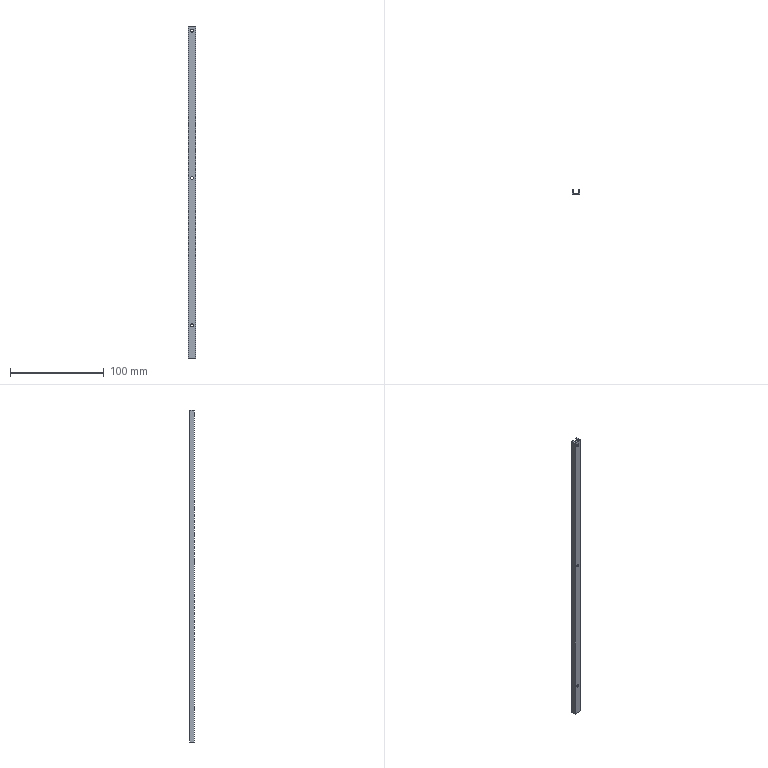Part | STEP file | 1 solid | 60 faces | box 8 x 5 x 355 mm | volume 6491 mm3 | cylinder 36 | plane 24 | commonest cylinder face diameters 0.2 x24 3 x6 5 x6